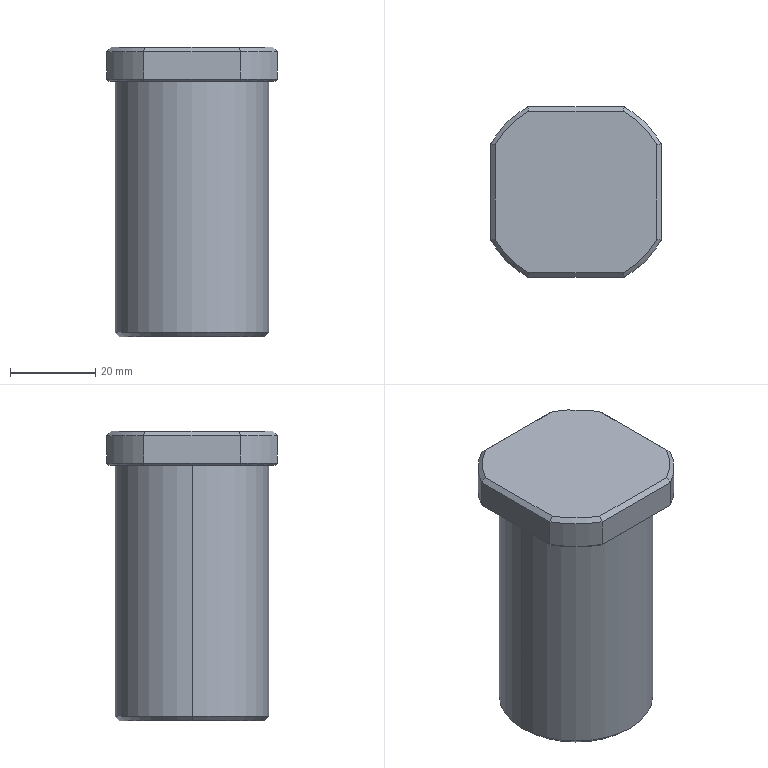Part | Creo | 1 solid | 41 faces | box 40 x 40 x 68 mm | volume 67467 mm3 | cone 16 | plane 15 | cylinder 10 | commonest cylinder face diameters 46 x4 13.8 x2 16 x2 36 x2
STEP:
#1=CARTESIAN_POINT('',(0.,0.,0.));
#2=DIRECTION('',(0.,0.,1.));
#3=DIRECTION('',(1.,0.,0.));
#4=AXIS2_PLACEMENT_3D('',#1,#2,#3);
#5=CARTESIAN_POINT('',(11.358,-20.,-233.));
#6=VERTEX_POINT('',#5);
#7=CARTESIAN_POINT('',(11.358,-20.,-226.5));
#8=VERTEX_POINT('',#7);
#9=CARTESIAN_POINT('',(11.358,-20.,-233.));
#10=DIRECTION('',(0.,0.,1.));
#11=VECTOR('',#10,6.5);
#12=LINE('',#9,#11);
#13=EDGE_CURVE('',#6,#8,#12,.T.);
#14=ORIENTED_EDGE('',*,*,#13,.T.);
#15=CARTESIAN_POINT('',(-11.358,-20.,-226.5));
#16=VERTEX_POINT('',#15);
#17=CARTESIAN_POINT('',(11.358,-20.,-226.5));
#18=DIRECTION('',(-1.,0.,0.));
#19=VECTOR('',#18,22.716);
#20=LINE('',#17,#19);
#21=EDGE_CURVE('',#8,#16,#20,.T.);
#22=ORIENTED_EDGE('',*,*,#21,.T.);
#23=CARTESIAN_POINT('',(-11.358,-20.,-233.));
#24=VERTEX_POINT('',#23);
#25=CARTESIAN_POINT('',(-11.358,-20.,-226.5));
#26=DIRECTION('',(0.,0.,-1.));
#27=VECTOR('',#26,6.5);
#28=LINE('',#25,#27);
#29=EDGE_CURVE('',#16,#24,#28,.T.);
#30=ORIENTED_EDGE('',*,*,#29,.T.);
#31=CARTESIAN_POINT('',(-11.358,-20.,-233.));
#32=DIRECTION('',(1.,0.,0.));
#33=VECTOR('',#32,22.716);
#34=LINE('',#31,#33);
#35=EDGE_CURVE('',#24,#6,#34,.T.);
#36=ORIENTED_EDGE('',*,*,#35,.T.);
#37=EDGE_LOOP('',(#14,#22,#30,#36));
#38=FACE_OUTER_BOUND('',#37,.F.);
#39=CARTESIAN_POINT('',(11.358,-20.,-233.5));
#40=DIRECTION('',(0.,1.,0.));
#41=DIRECTION('',(0.,0.,1.));
#42=AXIS2_PLACEMENT_3D('',#39,#40,#41);
#43=PLANE('',#42);
#44=ADVANCED_FACE('',(#38),#43,.T.);
#45=CARTESIAN_POINT('',(20.,-28.642,-226.5));
#46=VERTEX_POINT('',#45);
#47=CARTESIAN_POINT('',(20.,-28.642,-233.));
#48=VERTEX_POINT('',#47);
#49=CARTESIAN_POINT('',(20.,-28.642,-226.5));
#50=DIRECTION('',(0.,0.,-1.));
#51=VECTOR('',#50,6.5);
#52=LINE('',#49,#51);
#53=EDGE_CURVE('',#46,#48,#52,.T.);
#54=ORIENTED_EDGE('',*,*,#53,.F.);
#55=CARTESIAN_POINT('',(0.,-40.,-226.5));
#56=DIRECTION('',(0.,0.,1.));
#57=DIRECTION('',(0.8696,0.4938,0.));
#58=AXIS2_PLACEMENT_3D('',#55,#56,#57);
#59=CIRCLE('',#58,23.);
#60=EDGE_CURVE('',#46,#8,#59,.T.);
#61=ORIENTED_EDGE('',*,*,#60,.T.);
#62=ORIENTED_EDGE('',*,*,#13,.F.);
#63=CARTESIAN_POINT('',(0.,-40.,-233.));
#64=DIRECTION('',(0.,0.,-1.));
#65=DIRECTION('',(0.4938,0.8696,0.));
#66=AXIS2_PLACEMENT_3D('',#63,#64,#65);
#67=CIRCLE('',#66,23.);
#68=EDGE_CURVE('',#6,#48,#67,.T.);
#69=ORIENTED_EDGE('',*,*,#68,.T.);
#70=EDGE_LOOP('',(#54,#61,#62,#69));
#71=FACE_OUTER_BOUND('',#70,.F.);
#72=CARTESIAN_POINT('',(0.,-40.,-233.5));
#73=DIRECTION('',(0.,0.,1.));
#74=DIRECTION('',(1.,0.,0.));
#75=AXIS2_PLACEMENT_3D('',#72,#73,#74);
#76=CYLINDRICAL_SURFACE('',#75,23.);
#77=ADVANCED_FACE('',(#71),#76,.T.);
#78=CARTESIAN_POINT('',(20.,-51.358,-233.));
#79=VERTEX_POINT('',#78);
#80=CARTESIAN_POINT('',(20.,-51.358,-226.5));
#81=VERTEX_POINT('',#80);
#82=CARTESIAN_POINT('',(20.,-51.358,-233.));
#83=DIRECTION('',(0.,0.,1.));
#84=VECTOR('',#83,6.5);
#85=LINE('',#82,#84);
#86=EDGE_CURVE('',#79,#81,#85,.T.);
#87=ORIENTED_EDGE('',*,*,#86,.T.);
#88=CARTESIAN_POINT('',(20.,-51.358,-226.5));
#89=DIRECTION('',(0.,1.,0.));
#90=VECTOR('',#89,22.716);
#91=LINE('',#88,#90);
#92=EDGE_CURVE('',#81,#46,#91,.T.);
#93=ORIENTED_EDGE('',*,*,#92,.T.);
#94=ORIENTED_EDGE('',*,*,#53,.T.);
#95=CARTESIAN_POINT('',(20.,-28.642,-233.));
#96=DIRECTION('',(0.,-1.,0.));
#97=VECTOR('',#96,22.716);
#98=LINE('',#95,#97);
#99=EDGE_CURVE('',#48,#79,#98,.T.);
#100=ORIENTED_EDGE('',*,*,#99,.T.);
#101=EDGE_LOOP('',(#87,#93,#94,#100));
#102=FACE_OUTER_BOUND('',#101,.F.);
#103=CARTESIAN_POINT('',(20.,-51.358,-233.5));
#104=DIRECTION('',(1.,0.,0.));
#105=DIRECTION('',(0.,0.,-1.));
#106=AXIS2_PLACEMENT_3D('',#103,#104,#105);
#107=PLANE('',#106);
#108=ADVANCED_FACE('',(#102),#107,.T.);
#109=CARTESIAN_POINT('',(11.358,-60.,-226.5));
#110=VERTEX_POINT('',#109);
#111=CARTESIAN_POINT('',(11.358,-60.,-233.));
#112=VERTEX_POINT('',#111);
#113=CARTESIAN_POINT('',(11.358,-60.,-226.5));
#114=DIRECTION('',(0.,0.,-1.));
#115=VECTOR('',#114,6.5);
#116=LINE('',#113,#115);
#117=EDGE_CURVE('',#110,#112,#116,.T.);
#118=ORIENTED_EDGE('',*,*,#117,.F.);
#119=CARTESIAN_POINT('',(0.,-40.,-226.5));
#120=DIRECTION('',(0.,0.,1.));
#121=DIRECTION('',(0.4938,-0.8696,0.));
#122=AXIS2_PLACEMENT_3D('',#119,#120,#121);
#123=CIRCLE('',#122,23.);
#124=EDGE_CURVE('',#110,#81,#123,.T.);
#125=ORIENTED_EDGE('',*,*,#124,.T.);
#126=ORIENTED_EDGE('',*,*,#86,.F.);
#127=CARTESIAN_POINT('',(0.,-40.,-233.));
#128=DIRECTION('',(0.,0.,-1.));
#129=DIRECTION('',(0.8696,-0.4938,0.));
#130=AXIS2_PLACEMENT_3D('',#127,#128,#129);
#131=CIRCLE('',#130,23.);
#132=EDGE_CURVE('',#79,#112,#131,.T.);
#133=ORIENTED_EDGE('',*,*,#132,.T.);
#134=EDGE_LOOP('',(#118,#125,#126,#133));
#135=FACE_OUTER_BOUND('',#134,.F.);
#136=CARTESIAN_POINT('',(0.,-40.,-233.5));
#137=DIRECTION('',(0.,0.,1.));
#138=DIRECTION('',(1.,0.,0.));
#139=AXIS2_PLACEMENT_3D('',#136,#137,#138);
#140=CYLINDRICAL_SURFACE('',#139,23.);
#141=ADVANCED_FACE('',(#135),#140,.T.);
#142=CARTESIAN_POINT('',(-11.358,-60.,-233.));
#143=VERTEX_POINT('',#142);
#144=CARTESIAN_POINT('',(-11.358,-60.,-226.5));
#145=VERTEX_POINT('',#144);
#146=CARTESIAN_POINT('',(-11.358,-60.,-233.));
#147=DIRECTION('',(0.,0.,1.));
#148=VECTOR('',#147,6.5);
#149=LINE('',#146,#148);
#150=EDGE_CURVE('',#143,#145,#149,.T.);
#151=ORIENTED_EDGE('',*,*,#150,.T.);
#152=CARTESIAN_POINT('',(-11.358,-60.,-226.5));
#153=DIRECTION('',(1.,0.,0.));
#154=VECTOR('',#153,22.716);
#155=LINE('',#152,#154);
#156=EDGE_CURVE('',#145,#110,#155,.T.);
#157=ORIENTED_EDGE('',*,*,#156,.T.);
#158=ORIENTED_EDGE('',*,*,#117,.T.);
#159=CARTESIAN_POINT('',(11.358,-60.,-233.));
#160=DIRECTION('',(-1.,0.,0.));
#161=VECTOR('',#160,22.716);
#162=LINE('',#159,#161);
#163=EDGE_CURVE('',#112,#143,#162,.T.);
#164=ORIENTED_EDGE('',*,*,#163,.T.);
#165=EDGE_LOOP('',(#151,#157,#158,#164));
#166=FACE_OUTER_BOUND('',#165,.F.);
#167=CARTESIAN_POINT('',(-11.358,-60.,-233.5));
#168=DIRECTION('',(0.,-1.,0.));
#169=DIRECTION('',(0.,0.,-1.));
#170=AXIS2_PLACEMENT_3D('',#167,#168,#169);
#171=PLANE('',#170);
#172=ADVANCED_FACE('',(#166),#171,.T.);
#173=CARTESIAN_POINT('',(-20.,-51.358,-226.5));
#174=VERTEX_POINT('',#173);
#175=CARTESIAN_POINT('',(-20.,-51.358,-233.));
#176=VERTEX_POINT('',#175);
#177=CARTESIAN_POINT('',(-20.,-51.358,-226.5));
#178=DIRECTION('',(0.,0.,-1.));
#179=VECTOR('',#178,6.5);
#180=LINE('',#177,#179);
#181=EDGE_CURVE('',#174,#176,#180,.T.);
#182=ORIENTED_EDGE('',*,*,#181,.F.);
#183=CARTESIAN_POINT('',(0.,-40.,-226.5));
#184=DIRECTION('',(0.,0.,1.));
#185=DIRECTION('',(-0.8696,-0.4938,0.));
#186=AXIS2_PLACEMENT_3D('',#183,#184,#185);
#187=CIRCLE('',#186,23.);
#188=EDGE_CURVE('',#174,#145,#187,.T.);
#189=ORIENTED_EDGE('',*,*,#188,.T.);
#190=ORIENTED_EDGE('',*,*,#150,.F.);
#191=CARTESIAN_POINT('',(0.,-40.,-233.));
#192=DIRECTION('',(0.,0.,-1.));
#193=DIRECTION('',(-0.4938,-0.8696,0.));
#194=AXIS2_PLACEMENT_3D('',#191,#192,#193);
#195=CIRCLE('',#194,23.);
#196=EDGE_CURVE('',#143,#176,#195,.T.);
#197=ORIENTED_EDGE('',*,*,#196,.T.);
#198=EDGE_LOOP('',(#182,#189,#190,#197));
#199=FACE_OUTER_BOUND('',#198,.F.);
#200=CARTESIAN_POINT('',(0.,-40.,-233.5));
#201=DIRECTION('',(0.,0.,1.));
#202=DIRECTION('',(1.,0.,0.));
#203=AXIS2_PLACEMENT_3D('',#200,#201,#202);
#204=CYLINDRICAL_SURFACE('',#203,23.);
#205=ADVANCED_FACE('',(#199),#204,.T.);
#206=CARTESIAN_POINT('',(-20.,-28.642,-233.));
#207=VERTEX_POINT('',#206);
#208=CARTESIAN_POINT('',(-20.,-28.642,-226.5));
#209=VERTEX_POINT('',#208);
#210=CARTESIAN_POINT('',(-20.,-28.642,-233.));
#211=DIRECTION('',(0.,0.,1.));
#212=VECTOR('',#211,6.5);
#213=LINE('',#210,#212);
#214=EDGE_CURVE('',#207,#209,#213,.T.);
#215=ORIENTED_EDGE('',*,*,#214,.T.);
#216=CARTESIAN_POINT('',(-20.,-28.642,-226.5));
#217=DIRECTION('',(0.,-1.,0.));
#218=VECTOR('',#217,22.716);
#219=LINE('',#216,#218);
#220=EDGE_CURVE('',#209,#174,#219,.T.);
#221=ORIENTED_EDGE('',*,*,#220,.T.);
#222=ORIENTED_EDGE('',*,*,#181,.T.);
#223=CARTESIAN_POINT('',(-20.,-51.358,-233.));
#224=DIRECTION('',(0.,1.,0.));
#225=VECTOR('',#224,22.716);
#226=LINE('',#223,#225);
#227=EDGE_CURVE('',#176,#207,#226,.T.);
#228=ORIENTED_EDGE('',*,*,#227,.T.);
#229=EDGE_LOOP('',(#215,#221,#222,#228));
#230=FACE_OUTER_BOUND('',#229,.F.);
#231=CARTESIAN_POINT('',(-20.,-28.642,-233.5));
#232=DIRECTION('',(-1.,0.,0.));
#233=DIRECTION('',(0.,0.,1.));
#234=AXIS2_PLACEMENT_3D('',#231,#232,#233);
#235=PLANE('',#234);
#236=ADVANCED_FACE('',(#230),#235,.T.);
#237=ORIENTED_EDGE('',*,*,#29,.F.);
#238=CARTESIAN_POINT('',(0.,-40.,-226.5));
#239=DIRECTION('',(0.,0.,1.));
#240=DIRECTION('',(-0.4938,0.8696,0.));
#241=AXIS2_PLACEMENT_3D('',#238,#239,#240);
#242=CIRCLE('',#241,23.);
#243=EDGE_CURVE('',#16,#209,#242,.T.);
#244=ORIENTED_EDGE('',*,*,#243,.T.);
#245=ORIENTED_EDGE('',*,*,#214,.F.);
#246=CARTESIAN_POINT('',(0.,-40.,-233.));
#247=DIRECTION('',(0.,0.,-1.));
#248=DIRECTION('',(-0.8696,0.4938,0.));
#249=AXIS2_PLACEMENT_3D('',#246,#247,#248);
#250=CIRCLE('',#249,23.);
#251=EDGE_CURVE('',#207,#24,#250,.T.);
#252=ORIENTED_EDGE('',*,*,#251,.T.);
#253=EDGE_LOOP('',(#237,#244,#245,#252));
#254=FACE_OUTER_BOUND('',#253,.F.);
#255=CARTESIAN_POINT('',(0.,-40.,-233.5));
#256=DIRECTION('',(0.,0.,1.));
#257=DIRECTION('',(1.,0.,0.));
#258=AXIS2_PLACEMENT_3D('',#255,#256,#257);
#259=CYLINDRICAL_SURFACE('',#258,23.);
#260=ADVANCED_FACE('',(#254),#259,.T.);
#261=CARTESIAN_POINT('',(-19.,-28.909,-225.5));
#262=VERTEX_POINT('',#261);
#263=CARTESIAN_POINT('',(-19.,-28.909,-225.5));
#264=CARTESIAN_POINT('',(-19.111,-28.879,-225.611));
#265=CARTESIAN_POINT('',(-19.333,-28.82,-225.833));
#266=CARTESIAN_POINT('',(-19.667,-28.73,-226.167));
#267=CARTESIAN_POINT('',(-19.889,-28.672,-226.389));
#268=CARTESIAN_POINT('',(-20.,-28.642,-226.5));
#269=B_SPLINE_CURVE_WITH_KNOTS('',3,(#263,#264,#265,#266,#267,#268),.UNSPECIFIED.,.F.,.F.,(4,1,1,4),(0.,0.3333,0.6667,1.),.UNSPECIFIED.);
#270=EDGE_CURVE('',#262,#209,#269,.T.);
#271=ORIENTED_EDGE('',*,*,#270,.T.);
#272=ORIENTED_EDGE('',*,*,#243,.F.);
#273=CARTESIAN_POINT('',(-11.091,-21.,-225.5));
#274=VERTEX_POINT('',#273);
#275=CARTESIAN_POINT('',(-11.091,-21.,-225.5));
#276=CARTESIAN_POINT('',(-11.12,-20.89,-225.61));
#277=CARTESIAN_POINT('',(-11.18,-20.67,-225.83));
#278=CARTESIAN_POINT('',(-11.269,-20.337,-226.163));
#279=CARTESIAN_POINT('',(-11.328,-20.112,-226.388));
#280=CARTESIAN_POINT('',(-11.358,-20.,-226.5));
#281=B_SPLINE_CURVE_WITH_KNOTS('',3,(#275,#276,#277,#278,#279,#280),.UNSPECIFIED.,.F.,.F.,(4,1,1,4),(0.,0.3333,0.6667,1.),.UNSPECIFIED.);
#282=EDGE_CURVE('',#274,#16,#281,.T.);
#283=ORIENTED_EDGE('',*,*,#282,.F.);
#284=CARTESIAN_POINT('',(0.,-40.,-225.5));
#285=DIRECTION('',(0.,0.,1.));
#286=DIRECTION('',(-0.5041,0.8636,0.));
#287=AXIS2_PLACEMENT_3D('',#284,#285,#286);
#288=CIRCLE('',#287,22.);
#289=EDGE_CURVE('',#274,#262,#288,.T.);
#290=ORIENTED_EDGE('',*,*,#289,.T.);
#291=EDGE_LOOP('',(#271,#272,#283,#290));
#292=FACE_OUTER_BOUND('',#291,.F.);
#293=CARTESIAN_POINT('',(0.,-40.,-226.));
#294=DIRECTION('',(0.,0.,-1.));
#295=DIRECTION('',(-1.,0.,0.));
#296=AXIS2_PLACEMENT_3D('',#293,#294,#295);
#297=CONICAL_SURFACE('',#296,22.5,45.);
#298=ADVANCED_FACE('',(#292),#297,.T.);
#299=CARTESIAN_POINT('',(-19.,-51.091,-225.5));
#300=VERTEX_POINT('',#299);
#301=CARTESIAN_POINT('',(-19.,-51.091,-225.5));
#302=CARTESIAN_POINT('',(-19.11,-51.12,-225.61));
#303=CARTESIAN_POINT('',(-19.33,-51.18,-225.83));
#304=CARTESIAN_POINT('',(-19.663,-51.269,-226.163));
#305=CARTESIAN_POINT('',(-19.888,-51.328,-226.388));
#306=CARTESIAN_POINT('',(-20.,-51.358,-226.5));
#307=B_SPLINE_CURVE_WITH_KNOTS('',3,(#301,#302,#303,#304,#305,#306),.UNSPECIFIED.,.F.,.F.,(4,1,1,4),(0.,0.3333,0.6667,1.),.UNSPECIFIED.);
#308=EDGE_CURVE('',#300,#174,#307,.T.);
#309=ORIENTED_EDGE('',*,*,#308,.T.);
#310=ORIENTED_EDGE('',*,*,#220,.F.);
#311=ORIENTED_EDGE('',*,*,#270,.F.);
#312=CARTESIAN_POINT('',(-19.,-51.091,-225.5));
#313=DIRECTION('',(0.,1.,0.));
#314=VECTOR('',#313,22.181);
#315=LINE('',#312,#314);
#316=EDGE_CURVE('',#300,#262,#315,.T.);
#317=ORIENTED_EDGE('',*,*,#316,.F.);
#318=EDGE_LOOP('',(#309,#310,#311,#317));
#319=FACE_OUTER_BOUND('',#318,.F.);
#320=CARTESIAN_POINT('',(-19.,-40.,-225.5));
#321=DIRECTION('',(0.7071,0.,-0.7071));
#322=DIRECTION('',(-0.7071,0.,-0.7071));
#323=AXIS2_PLACEMENT_3D('',#320,#321,#322);
#324=PLANE('',#323);
#325=ADVANCED_FACE('',(#319),#324,.F.);
#326=ORIENTED_EDGE('',*,*,#308,.F.);
#327=CARTESIAN_POINT('',(-11.091,-59.,-225.5));
#328=VERTEX_POINT('',#327);
#329=CARTESIAN_POINT('',(0.,-40.,-225.5));
#330=DIRECTION('',(0.,0.,1.));
#331=DIRECTION('',(-0.8636,-0.5041,0.));
#332=AXIS2_PLACEMENT_3D('',#329,#330,#331);
#333=CIRCLE('',#332,22.);
#334=EDGE_CURVE('',#300,#328,#333,.T.);
#335=ORIENTED_EDGE('',*,*,#334,.T.);
#336=CARTESIAN_POINT('',(-11.358,-60.,-226.5));
#337=CARTESIAN_POINT('',(-11.328,-59.888,-226.388));
#338=CARTESIAN_POINT('',(-11.269,-59.663,-226.163));
#339=CARTESIAN_POINT('',(-11.18,-59.33,-225.83));
#340=CARTESIAN_POINT('',(-11.12,-59.11,-225.61));
#341=CARTESIAN_POINT('',(-11.091,-59.,-225.5));
#342=B_SPLINE_CURVE_WITH_KNOTS('',3,(#336,#337,#338,#339,#340,#341),.UNSPECIFIED.,.F.,.F.,(4,1,1,4),(0.,0.3333,0.6667,1.),.UNSPECIFIED.);
#343=EDGE_CURVE('',#145,#328,#342,.T.);
#344=ORIENTED_EDGE('',*,*,#343,.F.);
#345=ORIENTED_EDGE('',*,*,#188,.F.);
#346=EDGE_LOOP('',(#326,#335,#344,#345));
#347=FACE_OUTER_BOUND('',#346,.F.);
#348=CARTESIAN_POINT('',(0.,-40.,-226.));
#349=DIRECTION('',(0.,0.,-1.));
#350=DIRECTION('',(-1.,0.,0.));
#351=AXIS2_PLACEMENT_3D('',#348,#349,#350);
#352=CONICAL_SURFACE('',#351,22.5,45.);
#353=ADVANCED_FACE('',(#347),#352,.T.);
#354=CARTESIAN_POINT('',(19.,-28.909,-225.5));
#355=VERTEX_POINT('',#354);
#356=CARTESIAN_POINT('',(19.,-51.091,-225.5));
#357=VERTEX_POINT('',#356);
#358=CARTESIAN_POINT('',(19.,-28.909,-225.5));
#359=DIRECTION('',(0.,-1.,0.));
#360=VECTOR('',#359,22.181);
#361=LINE('',#358,#360);
#362=EDGE_CURVE('',#355,#357,#361,.T.);
#363=ORIENTED_EDGE('',*,*,#362,.T.);
#364=CARTESIAN_POINT('',(11.091,-59.,-225.5));
#365=VERTEX_POINT('',#364);
#366=CARTESIAN_POINT('',(0.,-40.,-225.5));
#367=DIRECTION('',(0.,0.,1.));
#368=DIRECTION('',(0.5041,-0.8636,0.));
#369=AXIS2_PLACEMENT_3D('',#366,#367,#368);
#370=CIRCLE('',#369,22.);
#371=EDGE_CURVE('',#365,#357,#370,.T.);
#372=ORIENTED_EDGE('',*,*,#371,.F.);
#373=CARTESIAN_POINT('',(11.091,-59.,-225.5));
#374=DIRECTION('',(-1.,0.,0.));
#375=VECTOR('',#374,22.181);
#376=LINE('',#373,#375);
#377=EDGE_CURVE('',#365,#328,#376,.T.);
#378=ORIENTED_EDGE('',*,*,#377,.T.);
#379=ORIENTED_EDGE('',*,*,#334,.F.);
#380=ORIENTED_EDGE('',*,*,#316,.T.);
#381=ORIENTED_EDGE('',*,*,#289,.F.);
#382=CARTESIAN_POINT('',(11.091,-21.,-225.5));
#383=VERTEX_POINT('',#382);
#384=CARTESIAN_POINT('',(-11.091,-21.,-225.5));
#385=DIRECTION('',(1.,0.,0.));
#386=VECTOR('',#385,22.181);
#387=LINE('',#384,#386);
#388=EDGE_CURVE('',#274,#383,#387,.T.);
#389=ORIENTED_EDGE('',*,*,#388,.T.);
#390=CARTESIAN_POINT('',(0.,-40.,-225.5));
#391=DIRECTION('',(0.,0.,1.));
#392=DIRECTION('',(0.8636,0.5041,0.));
#393=AXIS2_PLACEMENT_3D('',#390,#391,#392);
#394=CIRCLE('',#393,22.);
#395=EDGE_CURVE('',#355,#383,#394,.T.);
#396=ORIENTED_EDGE('',*,*,#395,.F.);
#397=EDGE_LOOP('',(#363,#372,#378,#379,#380,#381,#389,#396));
#398=FACE_OUTER_BOUND('',#397,.F.);
#399=CARTESIAN_POINT('',(0.,-40.,-225.5));
#400=DIRECTION('',(0.,0.,1.));
#401=DIRECTION('',(1.,0.,0.));
#402=AXIS2_PLACEMENT_3D('',#399,#400,#401);
#403=PLANE('',#402);
#404=ADVANCED_FACE('',(#398),#403,.T.);
#405=CARTESIAN_POINT('',(20.,-51.358,-226.5));
#406=CARTESIAN_POINT('',(19.888,-51.328,-226.388));
#407=CARTESIAN_POINT('',(19.663,-51.269,-226.163));
#408=CARTESIAN_POINT('',(19.33,-51.18,-225.83));
#409=CARTESIAN_POINT('',(19.11,-51.12,-225.61));
#410=CARTESIAN_POINT('',(19.,-51.091,-225.5));
#411=B_SPLINE_CURVE_WITH_KNOTS('',3,(#405,#406,#407,#408,#409,#410),.UNSPECIFIED.,.F.,.F.,(4,1,1,4),(0.,0.3333,0.6667,1.),.UNSPECIFIED.);
#412=EDGE_CURVE('',#81,#357,#411,.T.);
#413=ORIENTED_EDGE('',*,*,#412,.T.);
#414=ORIENTED_EDGE('',*,*,#362,.F.);
#415=CARTESIAN_POINT('',(20.,-28.642,-226.5));
#416=CARTESIAN_POINT('',(19.889,-28.672,-226.389));
#417=CARTESIAN_POINT('',(19.667,-28.73,-226.167));
#418=CARTESIAN_POINT('',(19.333,-28.82,-225.833));
#419=CARTESIAN_POINT('',(19.111,-28.879,-225.611));
#420=CARTESIAN_POINT('',(19.,-28.909,-225.5));
#421=B_SPLINE_CURVE_WITH_KNOTS('',3,(#415,#416,#417,#418,#419,#420),.UNSPECIFIED.,.F.,.F.,(4,1,1,4),(0.,0.3333,0.6667,1.),.UNSPECIFIED.);
#422=EDGE_CURVE('',#46,#355,#421,.T.);
#423=ORIENTED_EDGE('',*,*,#422,.F.);
#424=ORIENTED_EDGE('',*,*,#92,.F.);
#425=EDGE_LOOP('',(#413,#414,#423,#424));
#426=FACE_OUTER_BOUND('',#425,.F.);
#427=CARTESIAN_POINT('',(19.,-40.,-225.5));
#428=DIRECTION('',(-0.7071,0.,-0.7071));
#429=DIRECTION('',(-0.7071,0.,0.7071));
#430=AXIS2_PLACEMENT_3D('',#427,#428,#429);
#431=PLANE('',#430);
#432=ADVANCED_FACE('',(#426),#431,.F.);
#433=CARTESIAN_POINT('',(11.358,-60.,-226.5));
#434=CARTESIAN_POINT('',(11.328,-59.889,-226.389));
#435=CARTESIAN_POINT('',(11.27,-59.667,-226.167));
#436=CARTESIAN_POINT('',(11.18,-59.333,-225.833));
#437=CARTESIAN_POINT('',(11.121,-59.111,-225.611));
#438=CARTESIAN_POINT('',(11.091,-59.,-225.5));
#439=B_SPLINE_CURVE_WITH_KNOTS('',3,(#433,#434,#435,#436,#437,#438),.UNSPECIFIED.,.F.,.F.,(4,1,1,4),(0.,0.3333,0.6667,1.),.UNSPECIFIED.);
#440=EDGE_CURVE('',#110,#365,#439,.T.);
#441=ORIENTED_EDGE('',*,*,#440,.T.);
#442=ORIENTED_EDGE('',*,*,#371,.T.);
#443=ORIENTED_EDGE('',*,*,#412,.F.);
#444=ORIENTED_EDGE('',*,*,#124,.F.);
#445=EDGE_LOOP('',(#441,#442,#443,#444));
#446=FACE_OUTER_BOUND('',#445,.F.);
#447=CARTESIAN_POINT('',(0.,-40.,-226.));
#448=DIRECTION('',(0.,0.,-1.));
#449=DIRECTION('',(-1.,0.,0.));
#450=AXIS2_PLACEMENT_3D('',#447,#448,#449);
#451=CONICAL_SURFACE('',#450,22.5,45.);
#452=ADVANCED_FACE('',(#446),#451,.T.);
#453=ORIENTED_EDGE('',*,*,#343,.T.);
#454=ORIENTED_EDGE('',*,*,#377,.F.);
#455=ORIENTED_EDGE('',*,*,#440,.F.);
#456=ORIENTED_EDGE('',*,*,#156,.F.);
#457=EDGE_LOOP('',(#453,#454,#455,#456));
#458=FACE_OUTER_BOUND('',#457,.F.);
#459=CARTESIAN_POINT('',(0.,-59.,-225.5));
#460=DIRECTION('',(0.,0.7071,-0.7071));
#461=DIRECTION('',(0.,0.7071,0.7071));
#462=AXIS2_PLACEMENT_3D('',#459,#460,#461);
#463=PLANE('',#462);
#464=ADVANCED_FACE('',(#458),#463,.F.);
#465=ORIENTED_EDGE('',*,*,#422,.T.);
#466=ORIENTED_EDGE('',*,*,#395,.T.);
#467=CARTESIAN_POINT('',(11.091,-21.,-225.5));
#468=CARTESIAN_POINT('',(11.121,-20.889,-225.611));
#469=CARTESIAN_POINT('',(11.18,-20.667,-225.833));
#470=CARTESIAN_POINT('',(11.27,-20.333,-226.167));
#471=CARTESIAN_POINT('',(11.328,-20.111,-226.389));
#472=CARTESIAN_POINT('',(11.358,-20.,-226.5));
#473=B_SPLINE_CURVE_WITH_KNOTS('',3,(#467,#468,#469,#470,#471,#472),.UNSPECIFIED.,.F.,.F.,(4,1,1,4),(0.,0.3333,0.6667,1.),.UNSPECIFIED.);
#474=EDGE_CURVE('',#383,#8,#473,.T.);
#475=ORIENTED_EDGE('',*,*,#474,.T.);
#476=ORIENTED_EDGE('',*,*,#60,.F.);
#477=EDGE_LOOP('',(#465,#466,#475,#476));
#478=FACE_OUTER_BOUND('',#477,.F.);
#479=CARTESIAN_POINT('',(0.,-40.,-226.));
#480=DIRECTION('',(0.,0.,-1.));
#481=DIRECTION('',(-1.,0.,0.));
#482=AXIS2_PLACEMENT_3D('',#479,#480,#481);
#483=CONICAL_SURFACE('',#482,22.5,45.);
#484=ADVANCED_FACE('',(#478),#483,.T.);
#485=ORIENTED_EDGE('',*,*,#282,.T.);
#486=ORIENTED_EDGE('',*,*,#21,.F.);
#487=ORIENTED_EDGE('',*,*,#474,.F.);
#488=ORIENTED_EDGE('',*,*,#388,.F.);
#489=EDGE_LOOP('',(#485,#486,#487,#488));
#490=FACE_OUTER_BOUND('',#489,.F.);
#491=CARTESIAN_POINT('',(0.,-21.,-225.5));
#492=DIRECTION('',(0.,-0.7071,-0.7071));
#493=DIRECTION('',(0.,0.7071,-0.7071));
#494=AXIS2_PLACEMENT_3D('',#491,#492,#493);
#495=PLANE('',#494);
#496=ADVANCED_FACE('',(#490),#495,.F.);
#497=CARTESIAN_POINT('',(-11.225,-20.5,-233.5));
#498=VERTEX_POINT('',#497);
#499=CARTESIAN_POINT('',(-11.358,-20.,-233.));
#500=CARTESIAN_POINT('',(-11.343,-20.056,-233.056));
#501=CARTESIAN_POINT('',(-11.314,-20.167,-233.167));
#502=CARTESIAN_POINT('',(-11.269,-20.333,-233.333));
#503=CARTESIAN_POINT('',(-11.24,-20.444,-233.444));
#504=CARTESIAN_POINT('',(-11.225,-20.5,-233.5));
#505=B_SPLINE_CURVE_WITH_KNOTS('',3,(#499,#500,#501,#502,#503,#504),.UNSPECIFIED.,.F.,.F.,(4,1,1,4),(0.,0.3333,0.6667,1.),.UNSPECIFIED.);
#506=EDGE_CURVE('',#24,#498,#505,.T.);
#507=ORIENTED_EDGE('',*,*,#506,.F.);
#508=ORIENTED_EDGE('',*,*,#251,.F.);
#509=CARTESIAN_POINT('',(-19.5,-28.775,-233.5));
#510=VERTEX_POINT('',#509);
#511=CARTESIAN_POINT('',(-19.5,-28.775,-233.5));
#512=CARTESIAN_POINT('',(-19.556,-28.76,-233.444));
#513=CARTESIAN_POINT('',(-19.667,-28.731,-233.333));
#514=CARTESIAN_POINT('',(-19.833,-28.686,-233.167));
#515=CARTESIAN_POINT('',(-19.944,-28.657,-233.056));
#516=CARTESIAN_POINT('',(-20.,-28.642,-233.));
#517=B_SPLINE_CURVE_WITH_KNOTS('',3,(#511,#512,#513,#514,#515,#516),.UNSPECIFIED.,.F.,.F.,(4,1,1,4),(0.,0.3333,0.6667,1.),.UNSPECIFIED.);
#518=EDGE_CURVE('',#510,#207,#517,.T.);
#519=ORIENTED_EDGE('',*,*,#518,.F.);
#520=CARTESIAN_POINT('',(0.,-40.,-233.5));
#521=DIRECTION('',(0.,0.,-1.));
#522=DIRECTION('',(-0.8667,0.4989,0.));
#523=AXIS2_PLACEMENT_3D('',#520,#521,#522);
#524=CIRCLE('',#523,22.5);
#525=EDGE_CURVE('',#510,#498,#524,.T.);
#526=ORIENTED_EDGE('',*,*,#525,.T.);
#527=EDGE_LOOP('',(#507,#508,#519,#526));
#528=FACE_OUTER_BOUND('',#527,.F.);
#529=CARTESIAN_POINT('',(0.,-40.,-233.25));
#530=DIRECTION('',(0.,0.,1.));
#531=DIRECTION('',(1.,0.,0.));
#532=AXIS2_PLACEMENT_3D('',#529,#530,#531);
#533=CONICAL_SURFACE('',#532,22.75,45.);
#534=ADVANCED_FACE('',(#528),#533,.T.);
#535=CARTESIAN_POINT('',(11.225,-20.5,-233.5));
#536=VERTEX_POINT('',#535);
#537=CARTESIAN_POINT('',(11.225,-20.5,-233.5));
#538=CARTESIAN_POINT('',(11.24,-20.444,-233.444));
#539=CARTESIAN_POINT('',(11.269,-20.333,-233.333));
#540=CARTESIAN_POINT('',(11.314,-20.167,-233.167));
#541=CARTESIAN_POINT('',(11.343,-20.056,-233.056));
#542=CARTESIAN_POINT('',(11.358,-20.,-233.));
#543=B_SPLINE_CURVE_WITH_KNOTS('',3,(#537,#538,#539,#540,#541,#542),.UNSPECIFIED.,.F.,.F.,(4,1,1,4),(0.,0.3333,0.6667,1.),.UNSPECIFIED.);
#544=EDGE_CURVE('',#536,#6,#543,.T.);
#545=ORIENTED_EDGE('',*,*,#544,.T.);
#546=ORIENTED_EDGE('',*,*,#35,.F.);
#547=ORIENTED_EDGE('',*,*,#506,.T.);
#548=CARTESIAN_POINT('',(11.225,-20.5,-233.5));
#549=DIRECTION('',(-1.,0.,0.));
#550=VECTOR('',#549,22.45);
#551=LINE('',#548,#550);
#552=EDGE_CURVE('',#536,#498,#551,.T.);
#553=ORIENTED_EDGE('',*,*,#552,.F.);
#554=EDGE_LOOP('',(#545,#546,#547,#553));
#555=FACE_OUTER_BOUND('',#554,.F.);
#556=CARTESIAN_POINT('',(11.358,-20.,-233.));
#557=DIRECTION('',(0.,0.7071,-0.7071));
#558=DIRECTION('',(0.,0.7071,0.7071));
#559=AXIS2_PLACEMENT_3D('',#556,#557,#558);
#560=PLANE('',#559);
#561=ADVANCED_FACE('',(#555),#560,.T.);
#562=ORIENTED_EDGE('',*,*,#544,.F.);
#563=CARTESIAN_POINT('',(19.5,-28.775,-233.5));
#564=VERTEX_POINT('',#563);
#565=CARTESIAN_POINT('',(0.,-40.,-233.5));
#566=DIRECTION('',(0.,0.,-1.));
#567=DIRECTION('',(0.4989,0.8667,0.));
#568=AXIS2_PLACEMENT_3D('',#565,#566,#567);
#569=CIRCLE('',#568,22.5);
#570=EDGE_CURVE('',#536,#564,#569,.T.);
#571=ORIENTED_EDGE('',*,*,#570,.T.);
#572=CARTESIAN_POINT('',(20.,-28.642,-233.));
#573=CARTESIAN_POINT('',(19.944,-28.657,-233.056));
#574=CARTESIAN_POINT('',(19.833,-28.686,-233.167));
#575=CARTESIAN_POINT('',(19.667,-28.731,-233.333));
#576=CARTESIAN_POINT('',(19.556,-28.76,-233.444));
#577=CARTESIAN_POINT('',(19.5,-28.775,-233.5));
#578=B_SPLINE_CURVE_WITH_KNOTS('',3,(#572,#573,#574,#575,#576,#577),.UNSPECIFIED.,.F.,.F.,(4,1,1,4),(0.,0.3333,0.6667,1.),.UNSPECIFIED.);
#579=EDGE_CURVE('',#48,#564,#578,.T.);
#580=ORIENTED_EDGE('',*,*,#579,.F.);
#581=ORIENTED_EDGE('',*,*,#68,.F.);
#582=EDGE_LOOP('',(#562,#571,#580,#581));
#583=FACE_OUTER_BOUND('',#582,.F.);
#584=CARTESIAN_POINT('',(0.,-40.,-233.25));
#585=DIRECTION('',(0.,0.,1.));
#586=DIRECTION('',(1.,0.,0.));
#587=AXIS2_PLACEMENT_3D('',#584,#585,#586);
#588=CONICAL_SURFACE('',#587,22.75,45.);
#589=ADVANCED_FACE('',(#583),#588,.T.);
#590=CARTESIAN_POINT('',(19.5,-51.225,-233.5));
#591=VERTEX_POINT('',#590);
#592=CARTESIAN_POINT('',(11.225,-59.5,-233.5));
#593=VERTEX_POINT('',#592);
#594=CARTESIAN_POINT('',(0.,-40.,-233.5));
#595=DIRECTION('',(0.,0.,-1.));
#596=DIRECTION('',(0.8667,-0.4989,0.));
#597=AXIS2_PLACEMENT_3D('',#594,#595,#596);
#598=CIRCLE('',#597,22.5);
#599=EDGE_CURVE('',#591,#593,#598,.T.);
#600=ORIENTED_EDGE('',*,*,#599,.F.);
#601=CARTESIAN_POINT('',(19.5,-51.225,-233.5));
#602=DIRECTION('',(0.,1.,0.));
#603=VECTOR('',#602,22.45);
#604=LINE('',#601,#603);
#605=EDGE_CURVE('',#591,#564,#604,.T.);
#606=ORIENTED_EDGE('',*,*,#605,.T.);
#607=ORIENTED_EDGE('',*,*,#570,.F.);
#608=ORIENTED_EDGE('',*,*,#552,.T.);
#609=ORIENTED_EDGE('',*,*,#525,.F.);
#610=CARTESIAN_POINT('',(-19.5,-51.225,-233.5));
#611=VERTEX_POINT('',#610);
#612=CARTESIAN_POINT('',(-19.5,-28.775,-233.5));
#613=DIRECTION('',(0.,-1.,0.));
#614=VECTOR('',#613,22.45);
#615=LINE('',#612,#614);
#616=EDGE_CURVE('',#510,#611,#615,.T.);
#617=ORIENTED_EDGE('',*,*,#616,.T.);
#618=CARTESIAN_POINT('',(-11.225,-59.5,-233.5));
#619=VERTEX_POINT('',#618);
#620=CARTESIAN_POINT('',(0.,-40.,-233.5));
#621=DIRECTION('',(0.,0.,-1.));
#622=DIRECTION('',(-0.4989,-0.8667,0.));
#623=AXIS2_PLACEMENT_3D('',#620,#621,#622);
#624=CIRCLE('',#623,22.5);
#625=EDGE_CURVE('',#619,#611,#624,.T.);
#626=ORIENTED_EDGE('',*,*,#625,.F.);
#627=CARTESIAN_POINT('',(-11.225,-59.5,-233.5));
#628=DIRECTION('',(1.,0.,0.));
#629=VECTOR('',#628,22.45);
#630=LINE('',#627,#629);
#631=EDGE_CURVE('',#619,#593,#630,.T.);
#632=ORIENTED_EDGE('',*,*,#631,.T.);
#633=EDGE_LOOP('',(#600,#606,#607,#608,#609,#617,#626,#632));
#634=FACE_OUTER_BOUND('',#633,.F.);
#635=CARTESIAN_POINT('',(18.,-40.,-233.5));
#636=VERTEX_POINT('',#635);
#637=CARTESIAN_POINT('',(-18.,-40.,-233.5));
#638=VERTEX_POINT('',#637);
#639=CARTESIAN_POINT('',(0.,-40.,-233.5));
#640=DIRECTION('',(0.,0.,1.));
#641=DIRECTION('',(1.,0.,0.));
#642=AXIS2_PLACEMENT_3D('',#639,#640,#641);
#643=CIRCLE('',#642,18.);
#644=EDGE_CURVE('',#636,#638,#643,.T.);
#645=ORIENTED_EDGE('',*,*,#644,.F.);
#646=CARTESIAN_POINT('',(0.,-40.,-233.5));
#647=DIRECTION('',(0.,0.,1.));
#648=DIRECTION('',(-1.,0.,0.));
#649=AXIS2_PLACEMENT_3D('',#646,#647,#648);
#650=CIRCLE('',#649,18.);
#651=EDGE_CURVE('',#638,#636,#650,.T.);
#652=ORIENTED_EDGE('',*,*,#651,.F.);
#653=EDGE_LOOP('',(#645,#652));
#654=FACE_BOUND('',#653,.F.);
#655=CARTESIAN_POINT('',(0.,-40.,-233.5));
#656=DIRECTION('',(0.,0.,1.));
#657=DIRECTION('',(1.,0.,0.));
#658=AXIS2_PLACEMENT_3D('',#655,#656,#657);
#659=PLANE('',#658);
#660=ADVANCED_FACE('',(#634,#654),#659,.F.);
#661=CARTESIAN_POINT('',(19.5,-51.225,-233.5));
#662=CARTESIAN_POINT('',(19.556,-51.24,-233.444));
#663=CARTESIAN_POINT('',(19.667,-51.269,-233.333));
#664=CARTESIAN_POINT('',(19.833,-51.314,-233.167));
#665=CARTESIAN_POINT('',(19.944,-51.343,-233.056));
#666=CARTESIAN_POINT('',(20.,-51.358,-233.));
#667=B_SPLINE_CURVE_WITH_KNOTS('',3,(#661,#662,#663,#664,#665,#666),.UNSPECIFIED.,.F.,.F.,(4,1,1,4),(0.,0.3333,0.6667,1.),.UNSPECIFIED.);
#668=EDGE_CURVE('',#591,#79,#667,.T.);
#669=ORIENTED_EDGE('',*,*,#668,.F.);
#670=ORIENTED_EDGE('',*,*,#599,.T.);
#671=CARTESIAN_POINT('',(11.358,-60.,-233.));
#672=CARTESIAN_POINT('',(11.343,-59.944,-233.056));
#673=CARTESIAN_POINT('',(11.314,-59.833,-233.167));
#674=CARTESIAN_POINT('',(11.269,-59.667,-233.333));
#675=CARTESIAN_POINT('',(11.24,-59.556,-233.444));
#676=CARTESIAN_POINT('',(11.225,-59.5,-233.5));
#677=B_SPLINE_CURVE_WITH_KNOTS('',3,(#671,#672,#673,#674,#675,#676),.UNSPECIFIED.,.F.,.F.,(4,1,1,4),(0.,0.3333,0.6667,1.),.UNSPECIFIED.);
#678=EDGE_CURVE('',#112,#593,#677,.T.);
#679=ORIENTED_EDGE('',*,*,#678,.F.);
#680=ORIENTED_EDGE('',*,*,#132,.F.);
#681=EDGE_LOOP('',(#669,#670,#679,#680));
#682=FACE_OUTER_BOUND('',#681,.F.);
#683=CARTESIAN_POINT('',(0.,-40.,-233.25));
#684=DIRECTION('',(0.,0.,1.));
#685=DIRECTION('',(1.,0.,0.));
#686=AXIS2_PLACEMENT_3D('',#683,#684,#685);
#687=CONICAL_SURFACE('',#686,22.75,45.);
#688=ADVANCED_FACE('',(#682),#687,.T.);
#689=ORIENTED_EDGE('',*,*,#579,.T.);
#690=ORIENTED_EDGE('',*,*,#605,.F.);
#691=ORIENTED_EDGE('',*,*,#668,.T.);
#692=ORIENTED_EDGE('',*,*,#99,.F.);
#693=EDGE_LOOP('',(#689,#690,#691,#692));
#694=FACE_OUTER_BOUND('',#693,.F.);
#695=CARTESIAN_POINT('',(20.,-51.358,-233.));
#696=DIRECTION('',(0.7071,0.,-0.7071));
#697=DIRECTION('',(-0.7071,0.,-0.7071));
#698=AXIS2_PLACEMENT_3D('',#695,#696,#697);
#699=PLANE('',#698);
#700=ADVANCED_FACE('',(#694),#699,.T.);
#701=CARTESIAN_POINT('',(-11.225,-59.5,-233.5));
#702=CARTESIAN_POINT('',(-11.24,-59.556,-233.444));
#703=CARTESIAN_POINT('',(-11.269,-59.667,-233.333));
#704=CARTESIAN_POINT('',(-11.314,-59.833,-233.167));
#705=CARTESIAN_POINT('',(-11.343,-59.944,-233.056));
#706=CARTESIAN_POINT('',(-11.358,-60.,-233.));
#707=B_SPLINE_CURVE_WITH_KNOTS('',3,(#701,#702,#703,#704,#705,#706),.UNSPECIFIED.,.F.,.F.,(4,1,1,4),(0.,0.3333,0.6667,1.),.UNSPECIFIED.);
#708=EDGE_CURVE('',#619,#143,#707,.T.);
#709=ORIENTED_EDGE('',*,*,#708,.T.);
#710=ORIENTED_EDGE('',*,*,#163,.F.);
#711=ORIENTED_EDGE('',*,*,#678,.T.);
#712=ORIENTED_EDGE('',*,*,#631,.F.);
#713=EDGE_LOOP('',(#709,#710,#711,#712));
#714=FACE_OUTER_BOUND('',#713,.F.);
#715=CARTESIAN_POINT('',(-11.358,-60.,-233.));
#716=DIRECTION('',(0.,-0.7071,-0.7071));
#717=DIRECTION('',(0.,0.7071,-0.7071));
#718=AXIS2_PLACEMENT_3D('',#715,#716,#717);
#719=PLANE('',#718);
#720=ADVANCED_FACE('',(#714),#719,.T.);
#721=CARTESIAN_POINT('',(-20.,-51.358,-233.));
#722=CARTESIAN_POINT('',(-19.944,-51.343,-233.056));
#723=CARTESIAN_POINT('',(-19.833,-51.314,-233.167));
#724=CARTESIAN_POINT('',(-19.667,-51.269,-233.333));
#725=CARTESIAN_POINT('',(-19.556,-51.24,-233.444));
#726=CARTESIAN_POINT('',(-19.5,-51.225,-233.5));
#727=B_SPLINE_CURVE_WITH_KNOTS('',3,(#721,#722,#723,#724,#725,#726),.UNSPECIFIED.,.F.,.F.,(4,1,1,4),(0.,0.3333,0.6667,1.),.UNSPECIFIED.);
#728=EDGE_CURVE('',#176,#611,#727,.T.);
#729=ORIENTED_EDGE('',*,*,#728,.F.);
#730=ORIENTED_EDGE('',*,*,#196,.F.);
#731=ORIENTED_EDGE('',*,*,#708,.F.);
#732=ORIENTED_EDGE('',*,*,#625,.T.);
#733=EDGE_LOOP('',(#729,#730,#731,#732));
#734=FACE_OUTER_BOUND('',#733,.F.);
#735=CARTESIAN_POINT('',(0.,-40.,-233.25));
#736=DIRECTION('',(0.,0.,1.));
#737=DIRECTION('',(1.,0.,0.));
#738=AXIS2_PLACEMENT_3D('',#735,#736,#737);
#739=CONICAL_SURFACE('',#738,22.75,45.);
#740=ADVANCED_FACE('',(#734),#739,.T.);
#741=ORIENTED_EDGE('',*,*,#518,.T.);
#742=ORIENTED_EDGE('',*,*,#227,.F.);
#743=ORIENTED_EDGE('',*,*,#728,.T.);
#744=ORIENTED_EDGE('',*,*,#616,.F.);
#745=EDGE_LOOP('',(#741,#742,#743,#744));
#746=FACE_OUTER_BOUND('',#745,.F.);
#747=CARTESIAN_POINT('',(-20.,-28.642,-233.));
#748=DIRECTION('',(-0.7071,0.,-0.7071));
#749=DIRECTION('',(-0.7071,0.,0.7071));
#750=AXIS2_PLACEMENT_3D('',#747,#748,#749);
#751=PLANE('',#750);
#752=ADVANCED_FACE('',(#746),#751,.T.);
#753=CARTESIAN_POINT('',(-18.,-40.,-292.5));
#754=VERTEX_POINT('',#753);
#755=CARTESIAN_POINT('',(18.,-40.,-292.5));
#756=VERTEX_POINT('',#755);
#757=CARTESIAN_POINT('',(0.,-40.,-292.5));
#758=DIRECTION('',(0.,0.,-1.));
#759=DIRECTION('',(-1.,0.,0.));
#760=AXIS2_PLACEMENT_3D('',#757,#758,#759);
#761=CIRCLE('',#760,18.);
#762=EDGE_CURVE('',#754,#756,#761,.T.);
#763=ORIENTED_EDGE('',*,*,#762,.T.);
#764=CARTESIAN_POINT('',(18.,-40.,-292.5));
#765=DIRECTION('',(0.,0.,1.));
#766=VECTOR('',#765,59.);
#767=LINE('',#764,#766);
#768=EDGE_CURVE('',#756,#636,#767,.T.);
#769=ORIENTED_EDGE('',*,*,#768,.T.);
#770=ORIENTED_EDGE('',*,*,#644,.T.);
#771=CARTESIAN_POINT('',(-18.,-40.,-292.5));
#772=DIRECTION('',(0.,0.,1.));
#773=VECTOR('',#772,59.);
#774=LINE('',#771,#773);
#775=EDGE_CURVE('',#754,#638,#774,.T.);
#776=ORIENTED_EDGE('',*,*,#775,.F.);
#777=EDGE_LOOP('',(#763,#769,#770,#776));
#778=FACE_OUTER_BOUND('',#777,.F.);
#779=CARTESIAN_POINT('',(0.,-40.,-293.5));
#780=DIRECTION('',(0.,0.,1.));
#781=DIRECTION('',(1.,0.,0.));
#782=AXIS2_PLACEMENT_3D('',#779,#780,#781);
#783=CYLINDRICAL_SURFACE('',#782,18.);
#784=ADVANCED_FACE('',(#778),#783,.T.);
#785=CARTESIAN_POINT('',(-17.,-40.,-293.5));
#786=VERTEX_POINT('',#785);
#787=CARTESIAN_POINT('',(17.,-40.,-293.5));
#788=VERTEX_POINT('',#787);
#789=CARTESIAN_POINT('',(0.,-40.,-293.5));
#790=DIRECTION('',(0.,0.,-1.));
#791=DIRECTION('',(-1.,0.,0.));
#792=AXIS2_PLACEMENT_3D('',#789,#790,#791);
#793=CIRCLE('',#792,17.);
#794=EDGE_CURVE('',#786,#788,#793,.T.);
#795=ORIENTED_EDGE('',*,*,#794,.T.);
#796=CARTESIAN_POINT('',(17.,-40.,-293.5));
#797=DIRECTION('',(0.7071,0.,0.7071));
#798=VECTOR('',#797,1.414);
#799=LINE('',#796,#798);
#800=EDGE_CURVE('',#788,#756,#799,.T.);
#801=ORIENTED_EDGE('',*,*,#800,.T.);
#802=ORIENTED_EDGE('',*,*,#762,.F.);
#803=CARTESIAN_POINT('',(-17.,-40.,-293.5));
#804=DIRECTION('',(-0.7071,0.,0.7071));
#805=VECTOR('',#804,1.414);
#806=LINE('',#803,#805);
#807=EDGE_CURVE('',#786,#754,#806,.T.);
#808=ORIENTED_EDGE('',*,*,#807,.F.);
#809=EDGE_LOOP('',(#795,#801,#802,#808));
#810=FACE_OUTER_BOUND('',#809,.F.);
#811=CARTESIAN_POINT('',(0.,-40.,-293.));
#812=DIRECTION('',(0.,0.,1.));
#813=DIRECTION('',(1.,0.,0.));
#814=AXIS2_PLACEMENT_3D('',#811,#812,#813);
#815=CONICAL_SURFACE('',#814,17.5,45.);
#816=ADVANCED_FACE('',(#810),#815,.T.);
#817=CARTESIAN_POINT('',(0.,-40.,-293.5));
#818=DIRECTION('',(0.,0.,-1.));
#819=DIRECTION('',(1.,0.,0.));
#820=AXIS2_PLACEMENT_3D('',#817,#818,#819);
#821=CIRCLE('',#820,17.);
#822=EDGE_CURVE('',#788,#786,#821,.T.);
#823=ORIENTED_EDGE('',*,*,#822,.F.);
#824=ORIENTED_EDGE('',*,*,#794,.F.);
#825=EDGE_LOOP('',(#823,#824));
#826=FACE_OUTER_BOUND('',#825,.F.);
#827=CARTESIAN_POINT('',(9.5,-40.,-293.5));
#828=VERTEX_POINT('',#827);
#829=CARTESIAN_POINT('',(-9.5,-40.,-293.5));
#830=VERTEX_POINT('',#829);
#831=CARTESIAN_POINT('',(0.,-40.,-293.5));
#832=DIRECTION('',(0.,0.,1.));
#833=DIRECTION('',(1.,0.,0.));
#834=AXIS2_PLACEMENT_3D('',#831,#832,#833);
#835=CIRCLE('',#834,9.5);
#836=EDGE_CURVE('',#828,#830,#835,.T.);
#837=ORIENTED_EDGE('',*,*,#836,.F.);
#838=CARTESIAN_POINT('',(0.,-40.,-293.5));
#839=DIRECTION('',(0.,0.,1.));
#840=DIRECTION('',(-1.,0.,0.));
#841=AXIS2_PLACEMENT_3D('',#838,#839,#840);
#842=CIRCLE('',#841,9.5);
#843=EDGE_CURVE('',#830,#828,#842,.T.);
#844=ORIENTED_EDGE('',*,*,#843,.F.);
#845=EDGE_LOOP('',(#837,#844));
#846=FACE_BOUND('',#845,.F.);
#847=CARTESIAN_POINT('',(0.,-40.,-293.5));
#848=DIRECTION('',(0.,0.,1.));
#849=DIRECTION('',(1.,0.,0.));
#850=AXIS2_PLACEMENT_3D('',#847,#848,#849);
#851=PLANE('',#850);
#852=ADVANCED_FACE('',(#826,#846),#851,.F.);
#853=CARTESIAN_POINT('',(8.,-40.,-292.));
#854=VERTEX_POINT('',#853);
#855=CARTESIAN_POINT('',(-8.,-40.,-292.));
#856=VERTEX_POINT('',#855);
#857=CARTESIAN_POINT('',(0.,-40.,-292.));
#858=DIRECTION('',(0.,0.,1.));
#859=DIRECTION('',(1.,0.,0.));
#860=AXIS2_PLACEMENT_3D('',#857,#858,#859);
#861=CIRCLE('',#860,8.);
#862=EDGE_CURVE('',#854,#856,#861,.T.);
#863=ORIENTED_EDGE('',*,*,#862,.F.);
#864=CARTESIAN_POINT('',(8.,-40.,-292.));
#865=DIRECTION('',(0.7071,0.,-0.7071));
#866=VECTOR('',#865,2.121);
#867=LINE('',#864,#866);
#868=EDGE_CURVE('',#854,#828,#867,.T.);
#869=ORIENTED_EDGE('',*,*,#868,.T.);
#870=ORIENTED_EDGE('',*,*,#836,.T.);
#871=CARTESIAN_POINT('',(-8.,-40.,-292.));
#872=DIRECTION('',(-0.7071,0.,-0.7071));
#873=VECTOR('',#872,2.121);
#874=LINE('',#871,#873);
#875=EDGE_CURVE('',#856,#830,#874,.T.);
#876=ORIENTED_EDGE('',*,*,#875,.F.);
#877=EDGE_LOOP('',(#863,#869,#870,#876));
#878=FACE_OUTER_BOUND('',#877,.F.);
#879=CARTESIAN_POINT('',(0.,-40.,-292.75));
#880=DIRECTION('',(0.,0.,-1.));
#881=DIRECTION('',(-1.,0.,0.));
#882=AXIS2_PLACEMENT_3D('',#879,#880,#881);
#883=CONICAL_SURFACE('',#882,8.75,45.);
#884=ADVANCED_FACE('',(#878),#883,.F.);
#885=ORIENTED_EDGE('',*,*,#862,.T.);
#886=CARTESIAN_POINT('',(-8.,-40.,-272.1));
#887=VERTEX_POINT('',#886);
#888=CARTESIAN_POINT('',(-8.,-40.,-292.));
#889=DIRECTION('',(0.,0.,1.));
#890=VECTOR('',#889,19.9);
#891=LINE('',#888,#890);
#892=EDGE_CURVE('',#856,#887,#891,.T.);
#893=ORIENTED_EDGE('',*,*,#892,.T.);
#894=CARTESIAN_POINT('',(8.,-40.,-272.1));
#895=VERTEX_POINT('',#894);
#896=CARTESIAN_POINT('',(0.,-40.,-272.1));
#897=DIRECTION('',(0.,0.,-1.));
#898=DIRECTION('',(-1.,0.,0.));
#899=AXIS2_PLACEMENT_3D('',#896,#897,#898);
#900=CIRCLE('',#899,8.);
#901=EDGE_CURVE('',#887,#895,#900,.T.);
#902=ORIENTED_EDGE('',*,*,#901,.T.);
#903=CARTESIAN_POINT('',(8.,-40.,-292.));
#904=DIRECTION('',(0.,0.,1.));
#905=VECTOR('',#904,19.9);
#906=LINE('',#903,#905);
#907=EDGE_CURVE('',#854,#895,#906,.T.);
#908=ORIENTED_EDGE('',*,*,#907,.F.);
#909=EDGE_LOOP('',(#885,#893,#902,#908));
#910=FACE_OUTER_BOUND('',#909,.F.);
#911=CARTESIAN_POINT('',(0.,-40.,-293.5));
#912=DIRECTION('',(0.,0.,1.));
#913=DIRECTION('',(1.,0.,0.));
#914=AXIS2_PLACEMENT_3D('',#911,#912,#913);
#915=CYLINDRICAL_SURFACE('',#914,8.);
#916=ADVANCED_FACE('',(#910),#915,.F.);
#917=CARTESIAN_POINT('',(0.,-40.,-292.));
#918=DIRECTION('',(0.,0.,1.));
#919=DIRECTION('',(-1.,0.,0.));
#920=AXIS2_PLACEMENT_3D('',#917,#918,#919);
#921=CIRCLE('',#920,8.);
#922=EDGE_CURVE('',#856,#854,#921,.T.);
#923=ORIENTED_EDGE('',*,*,#922,.T.);
#924=ORIENTED_EDGE('',*,*,#907,.T.);
#925=CARTESIAN_POINT('',(0.,-40.,-272.1));
#926=DIRECTION('',(0.,0.,-1.));
#927=DIRECTION('',(1.,0.,0.));
#928=AXIS2_PLACEMENT_3D('',#925,#926,#927);
#929=CIRCLE('',#928,8.);
#930=EDGE_CURVE('',#895,#887,#929,.T.);
#931=ORIENTED_EDGE('',*,*,#930,.T.);
#932=ORIENTED_EDGE('',*,*,#892,.F.);
#933=EDGE_LOOP('',(#923,#924,#931,#932));
#934=FACE_OUTER_BOUND('',#933,.F.);
#935=CARTESIAN_POINT('',(0.,-40.,-293.5));
#936=DIRECTION('',(0.,0.,1.));
#937=DIRECTION('',(1.,0.,0.));
#938=AXIS2_PLACEMENT_3D('',#935,#936,#937);
#939=CYLINDRICAL_SURFACE('',#938,8.);
#940=ADVANCED_FACE('',(#934),#939,.F.);
#941=ORIENTED_EDGE('',*,*,#922,.F.);
#942=ORIENTED_EDGE('',*,*,#875,.T.);
#943=ORIENTED_EDGE('',*,*,#843,.T.);
#944=ORIENTED_EDGE('',*,*,#868,.F.);
#945=EDGE_LOOP('',(#941,#942,#943,#944));
#946=FACE_OUTER_BOUND('',#945,.F.);
#947=CARTESIAN_POINT('',(0.,-40.,-292.75));
#948=DIRECTION('',(0.,0.,-1.));
#949=DIRECTION('',(-1.,0.,0.));
#950=AXIS2_PLACEMENT_3D('',#947,#948,#949);
#951=CONICAL_SURFACE('',#950,8.75,45.);
#952=ADVANCED_FACE('',(#946),#951,.F.);
#953=ORIENTED_EDGE('',*,*,#930,.F.);
#954=CARTESIAN_POINT('',(6.9,-40.,-271.));
#955=VERTEX_POINT('',#954);
#956=CARTESIAN_POINT('',(6.9,-40.,-271.));
#957=DIRECTION('',(0.7071,0.,-0.7071));
#958=VECTOR('',#957,1.556);
#959=LINE('',#956,#958);
#960=EDGE_CURVE('',#955,#895,#959,.T.);
#961=ORIENTED_EDGE('',*,*,#960,.F.);
#962=CARTESIAN_POINT('',(-6.9,-40.,-271.));
#963=VERTEX_POINT('',#962);
#964=CARTESIAN_POINT('',(0.,-40.,-271.));
#965=DIRECTION('',(0.,0.,1.));
#966=DIRECTION('',(-1.,0.,0.));
#967=AXIS2_PLACEMENT_3D('',#964,#965,#966);
#968=CIRCLE('',#967,6.9);
#969=EDGE_CURVE('',#963,#955,#968,.T.);
#970=ORIENTED_EDGE('',*,*,#969,.F.);
#971=CARTESIAN_POINT('',(-6.9,-40.,-271.));
#972=DIRECTION('',(-0.7071,0.,-0.7071));
#973=VECTOR('',#972,1.556);
#974=LINE('',#971,#973);
#975=EDGE_CURVE('',#963,#887,#974,.T.);
#976=ORIENTED_EDGE('',*,*,#975,.T.);
#977=EDGE_LOOP('',(#953,#961,#970,#976));
#978=FACE_OUTER_BOUND('',#977,.F.);
#979=CARTESIAN_POINT('',(0.,-40.,-271.55));
#980=DIRECTION('',(0.,0.,-1.));
#981=DIRECTION('',(-1.,0.,0.));
#982=AXIS2_PLACEMENT_3D('',#979,#980,#981);
#983=CONICAL_SURFACE('',#982,7.45,45.);
#984=ADVANCED_FACE('',(#978),#983,.F.);
#985=ORIENTED_EDGE('',*,*,#901,.F.);
#986=ORIENTED_EDGE('',*,*,#975,.F.);
#987=CARTESIAN_POINT('',(0.,-40.,-271.));
#988=DIRECTION('',(0.,0.,1.));
#989=DIRECTION('',(1.,0.,0.));
#990=AXIS2_PLACEMENT_3D('',#987,#988,#989);
#991=CIRCLE('',#990,6.9);
#992=EDGE_CURVE('',#955,#963,#991,.T.);
#993=ORIENTED_EDGE('',*,*,#992,.F.);
#994=ORIENTED_EDGE('',*,*,#960,.T.);
#995=EDGE_LOOP('',(#985,#986,#993,#994));
#996=FACE_OUTER_BOUND('',#995,.F.);
#997=CARTESIAN_POINT('',(0.,-40.,-271.55));
#998=DIRECTION('',(0.,0.,-1.));
#999=DIRECTION('',(-1.,0.,0.));
#1000=AXIS2_PLACEMENT_3D('',#997,#998,#999);
#1001=CONICAL_SURFACE('',#1000,7.45,45.);
#1002=ADVANCED_FACE('',(#996),#1001,.F.);
#1003=ORIENTED_EDGE('',*,*,#992,.T.);
#1004=CARTESIAN_POINT('',(-6.9,-40.,-267.5));
#1005=VERTEX_POINT('',#1004);
#1006=CARTESIAN_POINT('',(-6.9,-40.,-271.));
#1007=DIRECTION('',(0.,0.,1.));
#1008=VECTOR('',#1007,3.5);
#1009=LINE('',#1006,#1008);
#1010=EDGE_CURVE('',#963,#1005,#1009,.T.);
#1011=ORIENTED_EDGE('',*,*,#1010,.T.);
#1012=CARTESIAN_POINT('',(6.9,-40.,-267.5));
#1013=VERTEX_POINT('',#1012);
#1014=CARTESIAN_POINT('',(0.,-40.,-267.5));
#1015=DIRECTION('',(0.,0.,-1.));
#1016=DIRECTION('',(-1.,0.,0.));
#1017=AXIS2_PLACEMENT_3D('',#1014,#1015,#1016);
#1018=CIRCLE('',#1017,6.9);
#1019=EDGE_CURVE('',#1005,#1013,#1018,.T.);
#1020=ORIENTED_EDGE('',*,*,#1019,.T.);
#1021=CARTESIAN_POINT('',(6.9,-40.,-271.));
#1022=DIRECTION('',(0.,0.,1.));
#1023=VECTOR('',#1022,3.5);
#1024=LINE('',#1021,#1023);
#1025=EDGE_CURVE('',#955,#1013,#1024,.T.);
#1026=ORIENTED_EDGE('',*,*,#1025,.F.);
#1027=EDGE_LOOP('',(#1003,#1011,#1020,#1026));
#1028=FACE_OUTER_BOUND('',#1027,.F.);
#1029=CARTESIAN_POINT('',(0.,-40.,-267.5));
#1030=DIRECTION('',(0.,0.,1.));
#1031=DIRECTION('',(1.,0.,0.));
#1032=AXIS2_PLACEMENT_3D('',#1029,#1030,#1031);
#1033=CYLINDRICAL_SURFACE('',#1032,6.9);
#1034=ADVANCED_FACE('',(#1028),#1033,.F.);
#1035=ORIENTED_EDGE('',*,*,#969,.T.);
#1036=ORIENTED_EDGE('',*,*,#1025,.T.);
#1037=CARTESIAN_POINT('',(0.,-40.,-267.5));
#1038=DIRECTION('',(0.,0.,-1.));
#1039=DIRECTION('',(1.,0.,0.));
#1040=AXIS2_PLACEMENT_3D('',#1037,#1038,#1039);
#1041=CIRCLE('',#1040,6.9);
#1042=EDGE_CURVE('',#1013,#1005,#1041,.T.);
#1043=ORIENTED_EDGE('',*,*,#1042,.T.);
#1044=ORIENTED_EDGE('',*,*,#1010,.F.);
#1045=EDGE_LOOP('',(#1035,#1036,#1043,#1044));
#1046=FACE_OUTER_BOUND('',#1045,.F.);
#1047=CARTESIAN_POINT('',(0.,-40.,-267.5));
#1048=DIRECTION('',(0.,0.,1.));
#1049=DIRECTION('',(1.,0.,0.));
#1050=AXIS2_PLACEMENT_3D('',#1047,#1048,#1049);
#1051=CYLINDRICAL_SURFACE('',#1050,6.9);
#1052=ADVANCED_FACE('',(#1046),#1051,.F.);
#1053=ORIENTED_EDGE('',*,*,#1042,.F.);
#1054=CARTESIAN_POINT('',(0.,-40.,-263.354));
#1055=VERTEX_POINT('',#1054);
#1056=CARTESIAN_POINT('',(0.,-40.,-263.354));
#1057=DIRECTION('',(0.8572,0.,-0.515));
#1058=VECTOR('',#1057,8.05);
#1059=LINE('',#1056,#1058);
#1060=EDGE_CURVE('',#1055,#1013,#1059,.T.);
#1061=ORIENTED_EDGE('',*,*,#1060,.F.);
#1062=CARTESIAN_POINT('',(0.,-40.,-263.354));
#1063=DIRECTION('',(-0.8572,0.,-0.515));
#1064=VECTOR('',#1063,8.05);
#1065=LINE('',#1062,#1064);
#1066=EDGE_CURVE('',#1055,#1005,#1065,.T.);
#1067=ORIENTED_EDGE('',*,*,#1066,.T.);
#1068=EDGE_LOOP('',(#1053,#1061,#1067));
#1069=FACE_OUTER_BOUND('',#1068,.F.);
#1070=CARTESIAN_POINT('',(0.,-40.,-265.468));
#1071=DIRECTION('',(0.,0.,-1.));
#1072=DIRECTION('',(-1.,0.,0.));
#1073=AXIS2_PLACEMENT_3D('',#1070,#1071,#1072);
#1074=CONICAL_SURFACE('',#1073,3.519,59.);
#1075=ADVANCED_FACE('',(#1069),#1074,.F.);
#1076=ORIENTED_EDGE('',*,*,#1019,.F.);
#1077=ORIENTED_EDGE('',*,*,#1066,.F.);
#1078=ORIENTED_EDGE('',*,*,#1060,.T.);
#1079=EDGE_LOOP('',(#1076,#1077,#1078));
#1080=FACE_OUTER_BOUND('',#1079,.F.);
#1081=CARTESIAN_POINT('',(0.,-40.,-265.468));
#1082=DIRECTION('',(0.,0.,-1.));
#1083=DIRECTION('',(-1.,0.,0.));
#1084=AXIS2_PLACEMENT_3D('',#1081,#1082,#1083);
#1085=CONICAL_SURFACE('',#1084,3.519,59.);
#1086=ADVANCED_FACE('',(#1080),#1085,.F.);
#1087=ORIENTED_EDGE('',*,*,#822,.T.);
#1088=ORIENTED_EDGE('',*,*,#807,.T.);
#1089=CARTESIAN_POINT('',(0.,-40.,-292.5));
#1090=DIRECTION('',(0.,0.,-1.));
#1091=DIRECTION('',(1.,0.,0.));
#1092=AXIS2_PLACEMENT_3D('',#1089,#1090,#1091);
#1093=CIRCLE('',#1092,18.);
#1094=EDGE_CURVE('',#756,#754,#1093,.T.);
#1095=ORIENTED_EDGE('',*,*,#1094,.F.);
#1096=ORIENTED_EDGE('',*,*,#800,.F.);
#1097=EDGE_LOOP('',(#1087,#1088,#1095,#1096));
#1098=FACE_OUTER_BOUND('',#1097,.F.);
#1099=CARTESIAN_POINT('',(0.,-40.,-293.));
#1100=DIRECTION('',(0.,0.,1.));
#1101=DIRECTION('',(1.,0.,0.));
#1102=AXIS2_PLACEMENT_3D('',#1099,#1100,#1101);
#1103=CONICAL_SURFACE('',#1102,17.5,45.);
#1104=ADVANCED_FACE('',(#1098),#1103,.T.);
#1105=ORIENTED_EDGE('',*,*,#1094,.T.);
#1106=ORIENTED_EDGE('',*,*,#775,.T.);
#1107=ORIENTED_EDGE('',*,*,#651,.T.);
#1108=ORIENTED_EDGE('',*,*,#768,.F.);
#1109=EDGE_LOOP('',(#1105,#1106,#1107,#1108));
#1110=FACE_OUTER_BOUND('',#1109,.F.);
#1111=CARTESIAN_POINT('',(0.,-40.,-293.5));
#1112=DIRECTION('',(0.,0.,1.));
#1113=DIRECTION('',(1.,0.,0.));
#1114=AXIS2_PLACEMENT_3D('',#1111,#1112,#1113);
#1115=CYLINDRICAL_SURFACE('',#1114,18.);
#1116=ADVANCED_FACE('',(#1110),#1115,.T.);
#1117=CLOSED_SHELL('',(#44,#77,#108,#141,#172,#205,#236,#260,#298,#325,#353,#404,#432,#452,#464,#484,#496,#534,#561,#589,#660,#688,#700,#720,#740,#752,#784,#816,#852,#884,#916,#940,#952,#984,#1002,#1034,#1052,#1075,#1086,#1104,#1116));
#1118=MANIFOLD_SOLID_BREP('',#1117);
#1119=(LENGTH_UNIT()NAMED_UNIT(*)SI_UNIT(.MILLI.,.METRE.));
#1120=UNCERTAINTY_MEASURE_WITH_UNIT(LENGTH_MEASURE(0.008845),#1119,'','');
#1121=(NAMED_UNIT(*)PLANE_ANGLE_UNIT()SI_UNIT($,.RADIAN.));
#1122=PLANE_ANGLE_MEASURE_WITH_UNIT(PLANE_ANGLE_MEASURE(0.01745),#1121);
#1123=(CONVERSION_BASED_UNIT('DEGREE',#1122)NAMED_UNIT(*)PLANE_ANGLE_UNIT());
#1124=(NAMED_UNIT(*)SI_UNIT($,.STERADIAN.)SOLID_ANGLE_UNIT());
#1125=(GEOMETRIC_REPRESENTATION_CONTEXT(3)GLOBAL_UNCERTAINTY_ASSIGNED_CONTEXT((#1120))GLOBAL_UNIT_ASSIGNED_CONTEXT((#1119,#1123,#1124))REPRESENTATION_CONTEXT('',''));
#1126=ADVANCED_BREP_SHAPE_REPRESENTATION('',(#4,#1118),#1125);